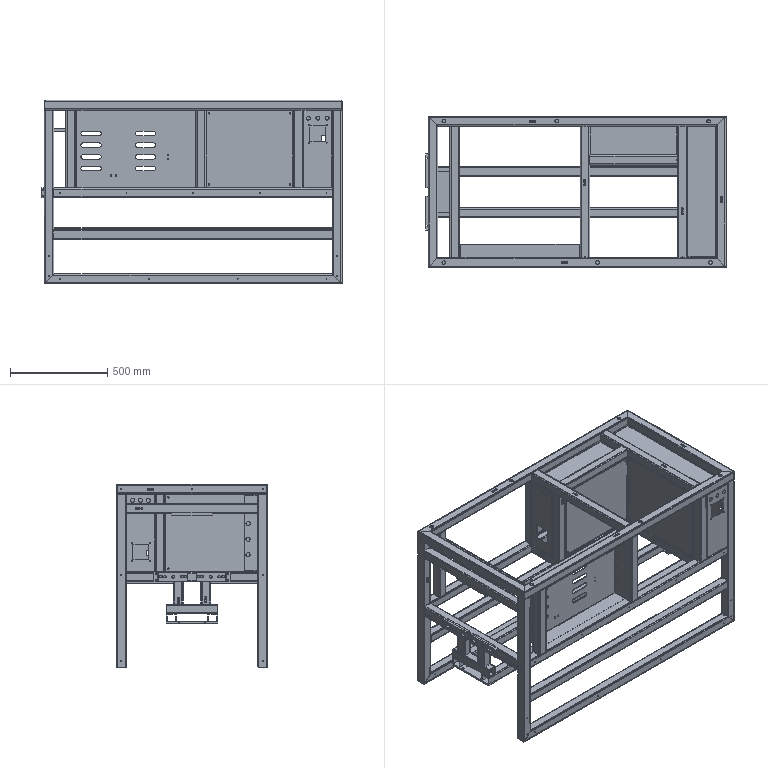Part | SolidWorks | 78 solids | 5232 faces | volume 20880442 mm3 | plane 2949 | spline 1296 | cylinder 945 | cone 42 | commonest cylinder face diameters 6 x182 12 x168 4.2 x96 0.4 x60 3.4 x56 8 x55